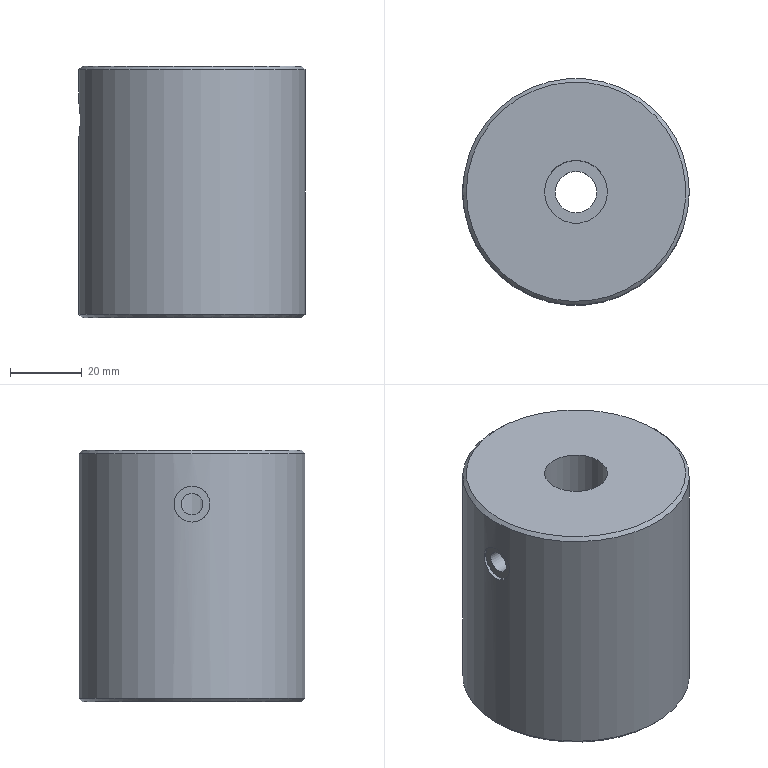Part | NX | features solid 2 | 1 solid | 11 faces | box 63 x 63 x 70 mm | volume 203219 mm3 | cylinder 5 | plane 4 | cone 2 | commonest cylinder face diameters 6 x1 10 x1 11.5 x1 17.5 x1 63 x1
STEP:
#1=CARTESIAN_POINT('',(-1365.5,-750.,-90.));
#2=VERTEX_POINT('',#1);
#3=CARTESIAN_POINT('',(-1335.,-750.,-90.));
#4=DIRECTION('',(0.,0.,1.));
#5=DIRECTION('',(-1.,0.,0.));
#6=AXIS2_PLACEMENT_3D('',#3,#4,#5);
#7=CIRCLE('',#6,30.5);
#8=EDGE_CURVE('',#2,#2,#7,.F.);
#9=ORIENTED_EDGE('',*,*,#8,.T.);
#10=EDGE_LOOP('',(#9));
#11=FACE_BOUND('',#10,.T.);
#12=CARTESIAN_POINT('',(-1340.75,-750.,-90.));
#13=VERTEX_POINT('',#12);
#14=CARTESIAN_POINT('',(-1335.,-750.,-90.));
#15=DIRECTION('',(0.,0.,1.));
#16=DIRECTION('',(-1.,0.,0.));
#17=AXIS2_PLACEMENT_3D('',#14,#15,#16);
#18=CIRCLE('',#17,5.75);
#19=EDGE_CURVE('',#13,#13,#18,.T.);
#20=ORIENTED_EDGE('',*,*,#19,.T.);
#21=EDGE_LOOP('',(#20));
#22=FACE_BOUND('',#21,.T.);
#23=CARTESIAN_POINT('',(-1335.,-750.,-90.));
#24=DIRECTION('',(0.,0.,1.));
#25=DIRECTION('',(-1.,0.,0.));
#26=AXIS2_PLACEMENT_3D('',#23,#24,#25);
#27=PLANE('',#26);
#28=ADVANCED_FACE('',(#11,#22),#27,.F.);
#29=CARTESIAN_POINT('',(-1343.75,-750.,-70.));
#30=VERTEX_POINT('',#29);
#31=CARTESIAN_POINT('',(-1335.,-750.,-70.));
#32=DIRECTION('',(0.,0.,1.));
#33=DIRECTION('',(-1.,0.,0.));
#34=AXIS2_PLACEMENT_3D('',#31,#32,#33);
#35=CIRCLE('',#34,8.75);
#36=EDGE_CURVE('',#30,#30,#35,.T.);
#37=ORIENTED_EDGE('',*,*,#36,.T.);
#38=EDGE_LOOP('',(#37));
#39=FACE_BOUND('',#38,.T.);
#40=CARTESIAN_POINT('',(-1340.75,-750.,-70.));
#41=VERTEX_POINT('',#40);
#42=CARTESIAN_POINT('',(-1335.,-750.,-70.));
#43=DIRECTION('',(0.,0.,1.));
#44=DIRECTION('',(-1.,0.,0.));
#45=AXIS2_PLACEMENT_3D('',#42,#43,#44);
#46=CIRCLE('',#45,5.75);
#47=EDGE_CURVE('',#41,#41,#46,.T.);
#48=ORIENTED_EDGE('',*,*,#47,.F.);
#49=EDGE_LOOP('',(#48));
#50=FACE_BOUND('',#49,.T.);
#51=CARTESIAN_POINT('',(-1335.,-750.,-70.));
#52=DIRECTION('',(0.,0.,1.));
#53=DIRECTION('',(-1.,0.,0.));
#54=AXIS2_PLACEMENT_3D('',#51,#52,#53);
#55=PLANE('',#54);
#56=ADVANCED_FACE('',(#39,#50),#55,.T.);
#57=CARTESIAN_POINT('',(-1365.5,-750.,-20.));
#58=VERTEX_POINT('',#57);
#59=CARTESIAN_POINT('',(-1335.,-750.,-20.));
#60=DIRECTION('',(0.,0.,1.));
#61=DIRECTION('',(-1.,0.,0.));
#62=AXIS2_PLACEMENT_3D('',#59,#60,#61);
#63=CIRCLE('',#62,30.5);
#64=EDGE_CURVE('',#58,#58,#63,.T.);
#65=ORIENTED_EDGE('',*,*,#64,.T.);
#66=EDGE_LOOP('',(#65));
#67=FACE_BOUND('',#66,.T.);
#68=CARTESIAN_POINT('',(-1326.25,-750.,-20.));
#69=VERTEX_POINT('',#68);
#70=CARTESIAN_POINT('',(-1335.,-750.,-20.));
#71=DIRECTION('',(0.,0.,-1.));
#72=DIRECTION('',(1.,0.,0.));
#73=AXIS2_PLACEMENT_3D('',#70,#71,#72);
#74=CIRCLE('',#73,8.75);
#75=EDGE_CURVE('',#69,#69,#74,.F.);
#76=ORIENTED_EDGE('',*,*,#75,.F.);
#77=EDGE_LOOP('',(#76));
#78=FACE_BOUND('',#77,.T.);
#79=CARTESIAN_POINT('',(-1335.,-750.,-20.));
#80=DIRECTION('',(0.,0.,1.));
#81=DIRECTION('',(-1.,0.,0.));
#82=AXIS2_PLACEMENT_3D('',#79,#80,#81);
#83=PLANE('',#82);
#84=ADVANCED_FACE('',(#67,#78),#83,.T.);
#85=CARTESIAN_POINT('',(-1366.5,-750.,-89.));
#86=VERTEX_POINT('',#85);
#87=CARTESIAN_POINT('',(-1335.,-750.,-89.));
#88=DIRECTION('',(0.,0.,1.));
#89=DIRECTION('',(-1.,0.,0.));
#90=AXIS2_PLACEMENT_3D('',#87,#88,#89);
#91=CIRCLE('',#90,31.5);
#92=EDGE_CURVE('',#86,#86,#91,.T.);
#93=ORIENTED_EDGE('',*,*,#92,.T.);
#94=EDGE_LOOP('',(#93));
#95=FACE_BOUND('',#94,.T.);
#96=CARTESIAN_POINT('',(-1366.5,-750.,-21.));
#97=VERTEX_POINT('',#96);
#98=CARTESIAN_POINT('',(-1335.,-750.,-21.));
#99=DIRECTION('',(0.,0.,1.));
#100=DIRECTION('',(-1.,0.,0.));
#101=AXIS2_PLACEMENT_3D('',#98,#99,#100);
#102=CIRCLE('',#101,31.5);
#103=EDGE_CURVE('',#97,#97,#102,.F.);
#104=ORIENTED_EDGE('',*,*,#103,.T.);
#105=EDGE_LOOP('',(#104));
#106=FACE_BOUND('',#105,.T.);
#107=CARTESIAN_POINT('',(-1366.499,-750.182,-39.997));
#108=VERTEX_POINT('',#107);
#109=CARTESIAN_POINT('',(-1366.279,-754.062,-38.77));
#110=CARTESIAN_POINT('',(-1366.599,-750.202,-40.539));
#111=CARTESIAN_POINT('',(-1366.323,-746.226,-39.056));
#112=CARTESIAN_POINT('',(-1366.001,-744.463,-35.207));
#113=CARTESIAN_POINT('',(-1366.28,-745.941,-31.227));
#114=CARTESIAN_POINT('',(-1366.598,-749.796,-29.464));
#115=CARTESIAN_POINT('',(-1366.324,-753.768,-30.938));
#116=CARTESIAN_POINT('',(-1366.001,-755.537,-34.793));
#117=CARTESIAN_POINT('',(-1366.279,-754.062,-38.77));
#118=CARTESIAN_POINT('',(-1366.599,-750.202,-40.539));
#119=CARTESIAN_POINT('',(-1366.323,-746.226,-39.056));
#120=B_SPLINE_CURVE_WITH_KNOTS('',3,(#109,#110,#111,#112,#113,#114,#115,#116,#117,#118,#119),.UNSPECIFIED.,.T.,.F.,(1,1,1,1,1,1,1,1,1,1,1,1,1,1,1),(-0.01174,-0.007828,-0.003914,0.,0.003914,0.007828,0.01174,0.01566,0.01957,0.02348,0.0274,0.03131,0.03522,0.03914,0.04305),.UNSPECIFIED.);
#121=EDGE_CURVE('',#108,#108,#120,.T.);
#122=ORIENTED_EDGE('',*,*,#121,.T.);
#123=EDGE_LOOP('',(#122));
#124=FACE_BOUND('',#123,.T.);
#125=CARTESIAN_POINT('',(-1335.,-750.,20.));
#126=DIRECTION('',(0.,0.,-1.));
#127=DIRECTION('',(1.,0.,0.));
#128=AXIS2_PLACEMENT_3D('',#125,#126,#127);
#129=CYLINDRICAL_SURFACE('',#128,31.5);
#130=ADVANCED_FACE('',(#95,#106,#124),#129,.T.);
#131=CARTESIAN_POINT('',(-1343.75,-750.034,-38.));
#132=VERTEX_POINT('',#131);
#133=CARTESIAN_POINT('',(-1343.484,-752.377,-37.324));
#134=CARTESIAN_POINT('',(-1343.878,-750.038,-38.325));
#135=CARTESIAN_POINT('',(-1343.502,-747.674,-37.374));
#136=CARTESIAN_POINT('',(-1343.083,-746.676,-35.042));
#137=CARTESIAN_POINT('',(-1343.484,-747.624,-32.674));
#138=CARTESIAN_POINT('',(-1343.878,-749.96,-31.676));
#139=CARTESIAN_POINT('',(-1343.502,-752.325,-32.623));
#140=CARTESIAN_POINT('',(-1343.083,-753.324,-34.962));
#141=CARTESIAN_POINT('',(-1343.484,-752.377,-37.324));
#142=CARTESIAN_POINT('',(-1343.878,-750.038,-38.325));
#143=CARTESIAN_POINT('',(-1343.502,-747.674,-37.374));
#144=B_SPLINE_CURVE_WITH_KNOTS('',3,(#133,#134,#135,#136,#137,#138,#139,#140,#141,#142,#143),.UNSPECIFIED.,.T.,.F.,(1,1,1,1,1,1,1,1,1,1,1,1,1,1,1),(-0.007088,-0.004725,-0.002363,0.,0.002363,0.004725,0.007088,0.009451,0.01181,0.01418,0.01654,0.0189,0.02126,0.02363,0.02599),.UNSPECIFIED.);
#145=EDGE_CURVE('',#132,#132,#144,.T.);
#146=ORIENTED_EDGE('',*,*,#145,.F.);
#147=EDGE_LOOP('',(#146));
#148=FACE_BOUND('',#147,.T.);
#149=ORIENTED_EDGE('',*,*,#75,.T.);
#150=EDGE_LOOP('',(#149));
#151=FACE_BOUND('',#150,.T.);
#152=ORIENTED_EDGE('',*,*,#36,.F.);
#153=EDGE_LOOP('',(#152));
#154=FACE_BOUND('',#153,.T.);
#155=CARTESIAN_POINT('',(-1335.,-750.,20.));
#156=DIRECTION('',(0.,0.,-1.));
#157=DIRECTION('',(1.,0.,0.));
#158=AXIS2_PLACEMENT_3D('',#155,#156,#157);
#159=CYLINDRICAL_SURFACE('',#158,8.75);
#160=ADVANCED_FACE('',(#148,#151,#154),#159,.F.);
#161=ORIENTED_EDGE('',*,*,#47,.T.);
#162=EDGE_LOOP('',(#161));
#163=FACE_BOUND('',#162,.T.);
#164=ORIENTED_EDGE('',*,*,#19,.F.);
#165=EDGE_LOOP('',(#164));
#166=FACE_BOUND('',#165,.T.);
#167=CARTESIAN_POINT('',(-1335.,-750.,-70.));
#168=DIRECTION('',(0.,0.,-1.));
#169=DIRECTION('',(1.,0.,0.));
#170=AXIS2_PLACEMENT_3D('',#167,#168,#169);
#171=CYLINDRICAL_SURFACE('',#170,5.75);
#172=ADVANCED_FACE('',(#163,#166),#171,.F.);
#173=CARTESIAN_POINT('',(-1365.5,-750.,-30.));
#174=VERTEX_POINT('',#173);
#175=CARTESIAN_POINT('',(-1365.5,-750.,-35.));
#176=DIRECTION('',(-1.,0.,0.));
#177=DIRECTION('',(0.,0.,1.));
#178=AXIS2_PLACEMENT_3D('',#175,#176,#177);
#179=CIRCLE('',#178,5.);
#180=EDGE_CURVE('',#174,#174,#179,.T.);
#181=ORIENTED_EDGE('',*,*,#180,.F.);
#182=EDGE_LOOP('',(#181));
#183=FACE_BOUND('',#182,.T.);
#184=ORIENTED_EDGE('',*,*,#121,.F.);
#185=EDGE_LOOP('',(#184));
#186=FACE_BOUND('',#185,.T.);
#187=CARTESIAN_POINT('',(-1354.,-750.,-35.));
#188=DIRECTION('',(-1.,0.,0.));
#189=DIRECTION('',(0.,0.,-1.));
#190=AXIS2_PLACEMENT_3D('',#187,#188,#189);
#191=CYLINDRICAL_SURFACE('',#190,5.);
#192=ADVANCED_FACE('',(#183,#186),#191,.F.);
#193=CARTESIAN_POINT('',(-1365.5,-750.,-32.));
#194=VERTEX_POINT('',#193);
#195=CARTESIAN_POINT('',(-1365.5,-750.,-35.));
#196=DIRECTION('',(1.,0.,0.));
#197=DIRECTION('',(0.,0.,1.));
#198=AXIS2_PLACEMENT_3D('',#195,#196,#197);
#199=CIRCLE('',#198,3.);
#200=EDGE_CURVE('',#194,#194,#199,.T.);
#201=ORIENTED_EDGE('',*,*,#200,.T.);
#202=EDGE_LOOP('',(#201));
#203=FACE_BOUND('',#202,.T.);
#204=ORIENTED_EDGE('',*,*,#180,.T.);
#205=EDGE_LOOP('',(#204));
#206=FACE_BOUND('',#205,.T.);
#207=CARTESIAN_POINT('',(-1365.5,-750.,-35.));
#208=DIRECTION('',(-1.,0.,0.));
#209=DIRECTION('',(0.,0.,-1.));
#210=AXIS2_PLACEMENT_3D('',#207,#208,#209);
#211=PLANE('',#210);
#212=ADVANCED_FACE('',(#203,#206),#211,.T.);
#213=ORIENTED_EDGE('',*,*,#145,.T.);
#214=EDGE_LOOP('',(#213));
#215=FACE_BOUND('',#214,.T.);
#216=ORIENTED_EDGE('',*,*,#200,.F.);
#217=EDGE_LOOP('',(#216));
#218=FACE_BOUND('',#217,.T.);
#219=CARTESIAN_POINT('',(-1354.,-750.,-35.));
#220=DIRECTION('',(1.,0.,0.));
#221=DIRECTION('',(0.,0.,1.));
#222=AXIS2_PLACEMENT_3D('',#219,#220,#221);
#223=CYLINDRICAL_SURFACE('',#222,3.);
#224=ADVANCED_FACE('',(#215,#218),#223,.F.);
#225=ORIENTED_EDGE('',*,*,#64,.F.);
#226=EDGE_LOOP('',(#225));
#227=FACE_BOUND('',#226,.T.);
#228=ORIENTED_EDGE('',*,*,#103,.F.);
#229=EDGE_LOOP('',(#228));
#230=FACE_BOUND('',#229,.T.);
#231=CARTESIAN_POINT('',(-1335.,-750.,-21.));
#232=DIRECTION('',(0.,0.,-1.));
#233=DIRECTION('',(1.,0.,0.));
#234=AXIS2_PLACEMENT_3D('',#231,#232,#233);
#235=CONICAL_SURFACE('',#234,31.5,0.7854);
#236=ADVANCED_FACE('',(#227,#230),#235,.T.);
#237=ORIENTED_EDGE('',*,*,#8,.F.);
#238=EDGE_LOOP('',(#237));
#239=FACE_BOUND('',#238,.T.);
#240=ORIENTED_EDGE('',*,*,#92,.F.);
#241=EDGE_LOOP('',(#240));
#242=FACE_BOUND('',#241,.T.);
#243=CARTESIAN_POINT('',(-1335.,-750.,-89.));
#244=DIRECTION('',(0.,0.,1.));
#245=DIRECTION('',(-1.,0.,0.));
#246=AXIS2_PLACEMENT_3D('',#243,#244,#245);
#247=CONICAL_SURFACE('',#246,31.5,0.7854);
#248=ADVANCED_FACE('',(#239,#242),#247,.T.);
#249=CLOSED_SHELL('',(#28,#56,#84,#130,#160,#172,#192,#212,#224,#236,#248));
#250=MANIFOLD_SOLID_BREP('',#249);
#251=(LENGTH_UNIT()NAMED_UNIT(*)SI_UNIT(.MILLI.,.METRE.));
#252=UNCERTAINTY_MEASURE_WITH_UNIT(LENGTH_MEASURE(0.0508),#251,'','');
#253=(NAMED_UNIT(*)PLANE_ANGLE_UNIT()SI_UNIT($,.RADIAN.));
#254=(NAMED_UNIT(*)SI_UNIT($,.STERADIAN.)SOLID_ANGLE_UNIT());
#255=(GEOMETRIC_REPRESENTATION_CONTEXT(3)GLOBAL_UNCERTAINTY_ASSIGNED_CONTEXT((#252))GLOBAL_UNIT_ASSIGNED_CONTEXT((#251,#253,#254))REPRESENTATION_CONTEXT('',''));
#256=ADVANCED_BREP_SHAPE_REPRESENTATION('',(#250),#255);